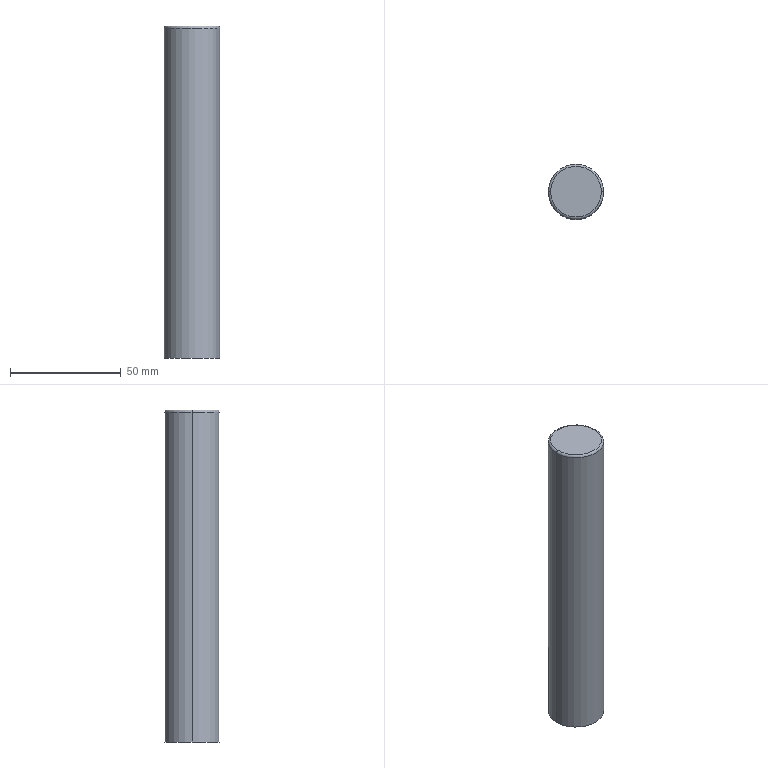Part | SolidWorks | features BaseBody 1 | 1 solid | 6 faces | box 25 x 25 x 150 mm | volume 73615 mm3 | torus 2 | cylinder 2 | plane 2 | commonest cylinder face diameters 25 x2
STEP:
#1=CARTESIAN_POINT('',(-154.5,65.,68.3));
#2=VERTEX_POINT('',#1);
#3=CARTESIAN_POINT('',(-177.5,65.,68.3));
#4=VERTEX_POINT('',#3);
#5=CARTESIAN_POINT('',(-166.,65.,68.3));
#6=DIRECTION('',(0.,0.,1.));
#7=DIRECTION('',(-1.,0.,0.));
#8=AXIS2_PLACEMENT_3D('',#5,#6,#7);
#9=CIRCLE('',#8,11.5);
#10=EDGE_CURVE('',#2,#4,#9,.T.);
#11=ORIENTED_EDGE('',*,*,#10,.F.);
#12=CARTESIAN_POINT('',(-153.5,65.,67.3));
#13=VERTEX_POINT('',#12);
#14=CARTESIAN_POINT('',(-154.5,65.,67.3));
#15=DIRECTION('',(0.,1.,0.));
#16=DIRECTION('',(-1.,0.,0.));
#17=AXIS2_PLACEMENT_3D('',#14,#15,#16);
#18=CIRCLE('',#17,1.);
#19=EDGE_CURVE('',#2,#13,#18,.T.);
#20=ORIENTED_EDGE('',*,*,#19,.T.);
#21=CARTESIAN_POINT('',(-178.5,65.,67.3));
#22=VERTEX_POINT('',#21);
#23=CARTESIAN_POINT('',(-166.,65.,67.3));
#24=DIRECTION('',(0.,0.,-1.));
#25=DIRECTION('',(-1.,0.,0.));
#26=AXIS2_PLACEMENT_3D('',#23,#24,#25);
#27=CIRCLE('',#26,12.5);
#28=EDGE_CURVE('',#22,#13,#27,.T.);
#29=ORIENTED_EDGE('',*,*,#28,.F.);
#30=CARTESIAN_POINT('',(-177.5,65.,67.3));
#31=DIRECTION('',(0.,-1.,0.));
#32=DIRECTION('',(0.,0.,-1.));
#33=AXIS2_PLACEMENT_3D('',#30,#31,#32);
#34=CIRCLE('',#33,1.);
#35=EDGE_CURVE('',#4,#22,#34,.T.);
#36=ORIENTED_EDGE('',*,*,#35,.F.);
#37=EDGE_LOOP('',(#11,#20,#29,#36));
#38=FACE_OUTER_BOUND('',#37,.T.);
#39=CARTESIAN_POINT('',(-166.,65.,67.3));
#40=DIRECTION('',(0.,0.,-1.));
#41=DIRECTION('',(-1.,0.,0.));
#42=AXIS2_PLACEMENT_3D('',#39,#40,#41);
#43=TOROIDAL_SURFACE('',#42,11.5,1.);
#44=ADVANCED_FACE('',(#38),#43,.T.);
#45=ORIENTED_EDGE('',*,*,#28,.T.);
#46=CARTESIAN_POINT('',(-153.5,65.,-81.7));
#47=VERTEX_POINT('',#46);
#48=CARTESIAN_POINT('',(-153.5,65.,78.3));
#49=DIRECTION('',(0.,0.,-1.));
#50=VECTOR('',#49,1000.);
#51=LINE('',#48,#50);
#52=EDGE_CURVE('',#13,#47,#51,.T.);
#53=ORIENTED_EDGE('',*,*,#52,.T.);
#54=CARTESIAN_POINT('',(-178.5,65.,-81.7));
#55=VERTEX_POINT('',#54);
#56=CARTESIAN_POINT('',(-166.,65.,-81.7));
#57=DIRECTION('',(0.,0.,-1.));
#58=DIRECTION('',(1.,0.,0.));
#59=AXIS2_PLACEMENT_3D('',#56,#57,#58);
#60=CIRCLE('',#59,12.5);
#61=EDGE_CURVE('',#55,#47,#60,.T.);
#62=ORIENTED_EDGE('',*,*,#61,.F.);
#63=CARTESIAN_POINT('',(-178.5,65.,78.3));
#64=DIRECTION('',(0.,0.,-1.));
#65=VECTOR('',#64,1000.);
#66=LINE('',#63,#65);
#67=EDGE_CURVE('',#22,#55,#66,.T.);
#68=ORIENTED_EDGE('',*,*,#67,.F.);
#69=EDGE_LOOP('',(#45,#53,#62,#68));
#70=FACE_OUTER_BOUND('',#69,.T.);
#71=CARTESIAN_POINT('',(-166.,65.,78.3));
#72=DIRECTION('',(0.,0.,-1.));
#73=DIRECTION('',(-1.,0.,0.));
#74=AXIS2_PLACEMENT_3D('',#71,#72,#73);
#75=CYLINDRICAL_SURFACE('',#74,12.5);
#76=ADVANCED_FACE('',(#70),#75,.T.);
#77=ORIENTED_EDGE('',*,*,#52,.F.);
#78=CARTESIAN_POINT('',(-166.,65.,67.3));
#79=DIRECTION('',(0.,0.,-1.));
#80=DIRECTION('',(-1.,0.,0.));
#81=AXIS2_PLACEMENT_3D('',#78,#79,#80);
#82=CIRCLE('',#81,12.5);
#83=EDGE_CURVE('',#13,#22,#82,.T.);
#84=ORIENTED_EDGE('',*,*,#83,.T.);
#85=ORIENTED_EDGE('',*,*,#67,.T.);
#86=CARTESIAN_POINT('',(-166.,65.,-81.7));
#87=DIRECTION('',(0.,0.,-1.));
#88=DIRECTION('',(1.,0.,0.));
#89=AXIS2_PLACEMENT_3D('',#86,#87,#88);
#90=CIRCLE('',#89,12.5);
#91=EDGE_CURVE('',#47,#55,#90,.T.);
#92=ORIENTED_EDGE('',*,*,#91,.F.);
#93=EDGE_LOOP('',(#77,#84,#85,#92));
#94=FACE_OUTER_BOUND('',#93,.T.);
#95=CARTESIAN_POINT('',(-166.,65.,78.3));
#96=DIRECTION('',(0.,0.,-1.));
#97=DIRECTION('',(-1.,0.,0.));
#98=AXIS2_PLACEMENT_3D('',#95,#96,#97);
#99=CYLINDRICAL_SURFACE('',#98,12.5);
#100=ADVANCED_FACE('',(#94),#99,.T.);
#101=CARTESIAN_POINT('',(-166.,65.,68.3));
#102=DIRECTION('',(0.,0.,1.));
#103=DIRECTION('',(-1.,0.,0.));
#104=AXIS2_PLACEMENT_3D('',#101,#102,#103);
#105=CIRCLE('',#104,11.5);
#106=EDGE_CURVE('',#4,#2,#105,.T.);
#107=ORIENTED_EDGE('',*,*,#106,.T.);
#108=ORIENTED_EDGE('',*,*,#10,.T.);
#109=EDGE_LOOP('',(#107,#108));
#110=FACE_OUTER_BOUND('',#109,.T.);
#111=CARTESIAN_POINT('',(-166.,65.,68.3));
#112=DIRECTION('',(0.,0.,-1.));
#113=DIRECTION('',(-1.,0.,0.));
#114=AXIS2_PLACEMENT_3D('',#111,#112,#113);
#115=PLANE('',#114);
#116=ADVANCED_FACE('',(#110),#115,.F.);
#117=ORIENTED_EDGE('',*,*,#61,.T.);
#118=ORIENTED_EDGE('',*,*,#91,.T.);
#119=EDGE_LOOP('',(#117,#118));
#120=FACE_OUTER_BOUND('',#119,.T.);
#121=CARTESIAN_POINT('',(-166.,65.,-81.7));
#122=DIRECTION('',(0.,0.,-1.));
#123=DIRECTION('',(-1.,0.,0.));
#124=AXIS2_PLACEMENT_3D('',#121,#122,#123);
#125=PLANE('',#124);
#126=ADVANCED_FACE('',(#120),#125,.T.);
#127=ORIENTED_EDGE('',*,*,#19,.F.);
#128=ORIENTED_EDGE('',*,*,#106,.F.);
#129=ORIENTED_EDGE('',*,*,#35,.T.);
#130=ORIENTED_EDGE('',*,*,#83,.F.);
#131=EDGE_LOOP('',(#127,#128,#129,#130));
#132=FACE_OUTER_BOUND('',#131,.T.);
#133=CARTESIAN_POINT('',(-166.,65.,67.3));
#134=DIRECTION('',(0.,0.,-1.));
#135=DIRECTION('',(-1.,0.,0.));
#136=AXIS2_PLACEMENT_3D('',#133,#134,#135);
#137=TOROIDAL_SURFACE('',#136,11.5,1.);
#138=ADVANCED_FACE('',(#132),#137,.T.);
#139=CLOSED_SHELL('',(#44,#76,#100,#116,#126,#138));
#140=MANIFOLD_SOLID_BREP('',#139);
#141=CARTESIAN_POINT('',(0.,0.,0.));
#142=DIRECTION('',(0.,0.,1.));
#143=DIRECTION('',(1.,0.,0.));
#144=AXIS2_PLACEMENT_3D('',#141,#142,#143);
#145=(LENGTH_UNIT()NAMED_UNIT(*)SI_UNIT(.MILLI.,.METRE.));
#146=UNCERTAINTY_MEASURE_WITH_UNIT(LENGTH_MEASURE(0.00001),#145,'','');
#147=(NAMED_UNIT(*)PLANE_ANGLE_UNIT()SI_UNIT($,.RADIAN.));
#148=(NAMED_UNIT(*)SI_UNIT($,.STERADIAN.)SOLID_ANGLE_UNIT());
#149=(GEOMETRIC_REPRESENTATION_CONTEXT(3)GLOBAL_UNCERTAINTY_ASSIGNED_CONTEXT((#146))GLOBAL_UNIT_ASSIGNED_CONTEXT((#145,#147,#148))REPRESENTATION_CONTEXT('',''));
#150=ADVANCED_BREP_SHAPE_REPRESENTATION('',(#140,#144),#149);